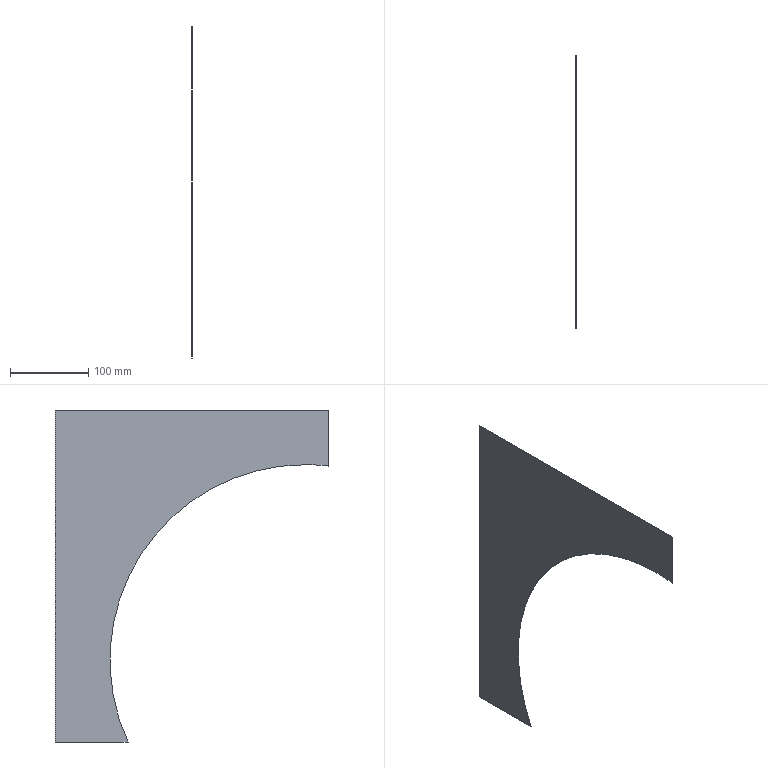Part | STEP file | 09-02 Inner base plate 1 | 1 solid | 8 faces | box 1 x 350 x 425 mm | volume 63574 mm3 | plane 6 | cylinder 2 | commonest cylinder face diameters 500 x2
STEP:
#1=CARTESIAN_POINT('',(0.,0.,0.));
#2=DIRECTION('',(0.,0.,1.));
#3=DIRECTION('',(1.,0.,0.));
#4=AXIS2_PLACEMENT_3D('',#1,#2,#3);
#5=CARTESIAN_POINT('',(0.,256.881,-425.));
#6=VERTEX_POINT('',#5);
#7=CARTESIAN_POINT('',(1.,256.881,-425.));
#8=VERTEX_POINT('',#7);
#9=CARTESIAN_POINT('',(0.5,256.881,-425.));
#10=DIRECTION('',(1.,0.,0.));
#11=VECTOR('',#10,1.);
#12=LINE('',#9,#11);
#13=CARTESIAN_POINT('',(1.,30.,-320.));
#14=DIRECTION('',(-1.,0.,0.));
#15=DIRECTION('',(0.,0.,1.));
#16=AXIS2_PLACEMENT_3D('',#13,#14,#15);
#17=CYLINDRICAL_SURFACE('',#16,250.);
#18=CARTESIAN_POINT('',(2.004,0.5));
#19=DIRECTION('',(0.,-1.));
#20=VECTOR('',#19,1.);
#21=LINE('',#18,#20);
#22=(GEOMETRIC_REPRESENTATION_CONTEXT(2)PARAMETRIC_REPRESENTATION_CONTEXT()REPRESENTATION_CONTEXT('',''));
#23=DEFINITIONAL_REPRESENTATION('',(#21),#22);
#24=PCURVE('',#17,#23);
#25=CARTESIAN_POINT('',(0.,256.881,-425.));
#26=DIRECTION('',(0.,0.,1.));
#27=DIRECTION('',(1.,0.,0.));
#28=AXIS2_PLACEMENT_3D('',#25,#26,#27);
#29=PLANE('',#28);
#30=CARTESIAN_POINT('',(0.5,0.));
#31=DIRECTION('',(1.,0.));
#32=VECTOR('',#31,1.);
#33=LINE('',#30,#32);
#34=(GEOMETRIC_REPRESENTATION_CONTEXT(2)PARAMETRIC_REPRESENTATION_CONTEXT()REPRESENTATION_CONTEXT('',''));
#35=DEFINITIONAL_REPRESENTATION('',(#33),#34);
#36=PCURVE('',#29,#35);
#37=SURFACE_CURVE('',#12,(#24,#36),.PCURVE_S1.);
#38=EDGE_CURVE('',#6,#8,#37,.T.);
#39=ORIENTED_EDGE('',*,*,#38,.F.);
#40=CARTESIAN_POINT('',(0.,30.,-70.));
#41=VERTEX_POINT('',#40);
#42=CARTESIAN_POINT('',(0.,30.,-320.));
#43=DIRECTION('',(-1.,0.,0.));
#44=DIRECTION('',(0.,0.,1.));
#45=AXIS2_PLACEMENT_3D('',#42,#43,#44);
#46=CIRCLE('',#45,250.);
#47=CARTESIAN_POINT('',(0.,1.));
#48=DIRECTION('',(1.,0.));
#49=VECTOR('',#48,1.);
#50=LINE('',#47,#49);
#51=(GEOMETRIC_REPRESENTATION_CONTEXT(2)PARAMETRIC_REPRESENTATION_CONTEXT()REPRESENTATION_CONTEXT('',''));
#52=DEFINITIONAL_REPRESENTATION('',(#50),#51);
#53=PCURVE('',#17,#52);
#54=CARTESIAN_POINT('',(0.,0.,0.));
#55=DIRECTION('',(1.,0.,0.));
#56=DIRECTION('',(0.,0.,-1.));
#57=AXIS2_PLACEMENT_3D('',#54,#55,#56);
#58=PLANE('',#57);
#59=CARTESIAN_POINT('',(70.,30.));
#60=CARTESIAN_POINT('',(70.,463.013));
#61=CARTESIAN_POINT('',(445.,246.506));
#62=CARTESIAN_POINT('',(820.,30.));
#63=CARTESIAN_POINT('',(445.,-186.506));
#64=CARTESIAN_POINT('',(70.,-403.013));
#65=CARTESIAN_POINT('',(70.,30.));
#66=(BOUNDED_CURVE()B_SPLINE_CURVE(2,(#59,#60,#61,#62,#63,#64,#65),.UNSPECIFIED.,.T.,.F.)B_SPLINE_CURVE_WITH_KNOTS((1,2,2,2,2,1),(-2.094,0.,2.094,4.189,6.283,8.378),.UNSPECIFIED.)CURVE()GEOMETRIC_REPRESENTATION_ITEM()RATIONAL_B_SPLINE_CURVE((1.,0.5,1.,0.5,1.,0.5,1.))REPRESENTATION_ITEM(''));
#67=(GEOMETRIC_REPRESENTATION_CONTEXT(2)PARAMETRIC_REPRESENTATION_CONTEXT()REPRESENTATION_CONTEXT('',''));
#68=DEFINITIONAL_REPRESENTATION('',(#66),#67);
#69=PCURVE('',#58,#68);
#70=SURFACE_CURVE('',#46,(#53,#69),.PCURVE_S1.);
#71=EDGE_CURVE('',#41,#6,#70,.T.);
#72=ORIENTED_EDGE('',*,*,#71,.F.);
#73=CARTESIAN_POINT('',(1.,30.,-70.));
#74=VERTEX_POINT('',#73);
#75=CARTESIAN_POINT('',(1.,30.,-70.));
#76=DIRECTION('',(-1.,0.,0.));
#77=VECTOR('',#76,1.);
#78=LINE('',#75,#77);
#79=CARTESIAN_POINT('',(0.,0.));
#80=DIRECTION('',(0.,1.));
#81=VECTOR('',#80,1.);
#82=LINE('',#79,#81);
#83=(GEOMETRIC_REPRESENTATION_CONTEXT(2)PARAMETRIC_REPRESENTATION_CONTEXT()REPRESENTATION_CONTEXT('',''));
#84=DEFINITIONAL_REPRESENTATION('',(#82),#83);
#85=PCURVE('',#17,#84);
#86=CARTESIAN_POINT('',(1.,30.,-320.));
#87=DIRECTION('',(-1.,0.,0.));
#88=DIRECTION('',(0.,0.,1.));
#89=AXIS2_PLACEMENT_3D('',#86,#87,#88);
#90=CYLINDRICAL_SURFACE('',#89,250.);
#91=CARTESIAN_POINT('',(6.283,0.));
#92=DIRECTION('',(0.,1.));
#93=VECTOR('',#92,1.);
#94=LINE('',#91,#93);
#95=(GEOMETRIC_REPRESENTATION_CONTEXT(2)PARAMETRIC_REPRESENTATION_CONTEXT()REPRESENTATION_CONTEXT('',''));
#96=DEFINITIONAL_REPRESENTATION('',(#94),#95);
#97=PCURVE('',#90,#96);
#98=SURFACE_CURVE('',#78,(#85,#97),.PCURVE_S1.);
#99=EDGE_CURVE('',#74,#41,#98,.T.);
#100=ORIENTED_EDGE('',*,*,#99,.F.);
#101=CARTESIAN_POINT('',(1.,30.,-320.));
#102=DIRECTION('',(1.,0.,0.));
#103=DIRECTION('',(0.,0.,1.));
#104=AXIS2_PLACEMENT_3D('',#101,#102,#103);
#105=CIRCLE('',#104,250.);
#106=CARTESIAN_POINT('',(6.283,0.));
#107=DIRECTION('',(-1.,0.));
#108=VECTOR('',#107,1.);
#109=LINE('',#106,#108);
#110=(GEOMETRIC_REPRESENTATION_CONTEXT(2)PARAMETRIC_REPRESENTATION_CONTEXT()REPRESENTATION_CONTEXT('',''));
#111=DEFINITIONAL_REPRESENTATION('',(#109),#110);
#112=PCURVE('',#17,#111);
#113=CARTESIAN_POINT('',(1.,0.,0.));
#114=DIRECTION('',(1.,0.,0.));
#115=DIRECTION('',(0.,0.,-1.));
#116=AXIS2_PLACEMENT_3D('',#113,#114,#115);
#117=PLANE('',#116);
#118=CARTESIAN_POINT('',(320.,30.));
#119=DIRECTION('',(-1.,0.));
#120=AXIS2_PLACEMENT_2D('',#118,#119);
#121=CIRCLE('',#120,250.);
#122=(GEOMETRIC_REPRESENTATION_CONTEXT(2)PARAMETRIC_REPRESENTATION_CONTEXT()REPRESENTATION_CONTEXT('',''));
#123=DEFINITIONAL_REPRESENTATION('',(#121),#122);
#124=PCURVE('',#117,#123);
#125=SURFACE_CURVE('',#105,(#112,#124),.PCURVE_S1.);
#126=EDGE_CURVE('',#8,#74,#125,.T.);
#127=ORIENTED_EDGE('',*,*,#126,.F.);
#128=EDGE_LOOP('',(#39,#72,#100,#127));
#129=FACE_BOUND('',#128,.F.);
#130=ADVANCED_FACE('',(#129),#17,.F.);
#131=CARTESIAN_POINT('',(0.,0.000000027,-71.807));
#132=VERTEX_POINT('',#131);
#133=CARTESIAN_POINT('',(0.,30.,-320.));
#134=DIRECTION('',(-1.,0.,0.));
#135=DIRECTION('',(0.,0.,1.));
#136=AXIS2_PLACEMENT_3D('',#133,#134,#135);
#137=CIRCLE('',#136,250.);
#138=CARTESIAN_POINT('',(0.,1.));
#139=DIRECTION('',(1.,0.));
#140=VECTOR('',#139,1.);
#141=LINE('',#138,#140);
#142=(GEOMETRIC_REPRESENTATION_CONTEXT(2)PARAMETRIC_REPRESENTATION_CONTEXT()REPRESENTATION_CONTEXT('',''));
#143=DEFINITIONAL_REPRESENTATION('',(#141),#142);
#144=PCURVE('',#90,#143);
#145=CARTESIAN_POINT('',(70.,30.));
#146=CARTESIAN_POINT('',(70.,463.013));
#147=CARTESIAN_POINT('',(445.,246.506));
#148=CARTESIAN_POINT('',(820.,30.));
#149=CARTESIAN_POINT('',(445.,-186.506));
#150=CARTESIAN_POINT('',(70.,-403.013));
#151=CARTESIAN_POINT('',(70.,30.));
#152=(BOUNDED_CURVE()B_SPLINE_CURVE(2,(#145,#146,#147,#148,#149,#150,#151),.UNSPECIFIED.,.T.,.F.)B_SPLINE_CURVE_WITH_KNOTS((1,2,2,2,2,1),(-2.094,0.,2.094,4.189,6.283,8.378),.UNSPECIFIED.)CURVE()GEOMETRIC_REPRESENTATION_ITEM()RATIONAL_B_SPLINE_CURVE((1.,0.5,1.,0.5,1.,0.5,1.))REPRESENTATION_ITEM(''));
#153=(GEOMETRIC_REPRESENTATION_CONTEXT(2)PARAMETRIC_REPRESENTATION_CONTEXT()REPRESENTATION_CONTEXT('',''));
#154=DEFINITIONAL_REPRESENTATION('',(#152),#153);
#155=PCURVE('',#58,#154);
#156=SURFACE_CURVE('',#137,(#144,#155),.PCURVE_S1.);
#157=EDGE_CURVE('',#132,#41,#156,.T.);
#158=ORIENTED_EDGE('',*,*,#157,.F.);
#159=CARTESIAN_POINT('',(1.,0.000000027,-71.807));
#160=VERTEX_POINT('',#159);
#161=CARTESIAN_POINT('',(0.5,0.000000053,-71.807));
#162=DIRECTION('',(-1.,0.,0.));
#163=VECTOR('',#162,1.);
#164=LINE('',#161,#163);
#165=CARTESIAN_POINT('',(6.163,0.5));
#166=DIRECTION('',(0.,1.));
#167=VECTOR('',#166,1.);
#168=LINE('',#165,#167);
#169=(GEOMETRIC_REPRESENTATION_CONTEXT(2)PARAMETRIC_REPRESENTATION_CONTEXT()REPRESENTATION_CONTEXT('',''));
#170=DEFINITIONAL_REPRESENTATION('',(#168),#169);
#171=PCURVE('',#90,#170);
#172=CARTESIAN_POINT('',(0.,0.,-71.807));
#173=DIRECTION('',(0.,1.,0.));
#174=DIRECTION('',(0.,0.,1.));
#175=AXIS2_PLACEMENT_3D('',#172,#173,#174);
#176=PLANE('',#175);
#177=CARTESIAN_POINT('',(0.000000006,0.5));
#178=DIRECTION('',(0.,-1.));
#179=VECTOR('',#178,1.);
#180=LINE('',#177,#179);
#181=(GEOMETRIC_REPRESENTATION_CONTEXT(2)PARAMETRIC_REPRESENTATION_CONTEXT()REPRESENTATION_CONTEXT('',''));
#182=DEFINITIONAL_REPRESENTATION('',(#180),#181);
#183=PCURVE('',#176,#182);
#184=SURFACE_CURVE('',#164,(#171,#183),.PCURVE_S1.);
#185=EDGE_CURVE('',#160,#132,#184,.T.);
#186=ORIENTED_EDGE('',*,*,#185,.F.);
#187=CARTESIAN_POINT('',(1.,30.,-320.));
#188=DIRECTION('',(1.,0.,0.));
#189=DIRECTION('',(0.,0.,1.));
#190=AXIS2_PLACEMENT_3D('',#187,#188,#189);
#191=CIRCLE('',#190,250.);
#192=CARTESIAN_POINT('',(6.283,0.));
#193=DIRECTION('',(-1.,0.));
#194=VECTOR('',#193,1.);
#195=LINE('',#192,#194);
#196=(GEOMETRIC_REPRESENTATION_CONTEXT(2)PARAMETRIC_REPRESENTATION_CONTEXT()REPRESENTATION_CONTEXT('',''));
#197=DEFINITIONAL_REPRESENTATION('',(#195),#196);
#198=PCURVE('',#90,#197);
#199=CARTESIAN_POINT('',(320.,30.));
#200=DIRECTION('',(-1.,0.));
#201=AXIS2_PLACEMENT_2D('',#199,#200);
#202=CIRCLE('',#201,250.);
#203=(GEOMETRIC_REPRESENTATION_CONTEXT(2)PARAMETRIC_REPRESENTATION_CONTEXT()REPRESENTATION_CONTEXT('',''));
#204=DEFINITIONAL_REPRESENTATION('',(#202),#203);
#205=PCURVE('',#117,#204);
#206=SURFACE_CURVE('',#191,(#198,#205),.PCURVE_S1.);
#207=EDGE_CURVE('',#74,#160,#206,.T.);
#208=ORIENTED_EDGE('',*,*,#207,.F.);
#209=ORIENTED_EDGE('',*,*,#99,.T.);
#210=EDGE_LOOP('',(#158,#186,#208,#209));
#211=FACE_BOUND('',#210,.F.);
#212=ADVANCED_FACE('',(#211),#90,.F.);
#213=CARTESIAN_POINT('',(0.,350.,-425.));
#214=VERTEX_POINT('',#213);
#215=CARTESIAN_POINT('',(0.,350.,0.));
#216=VERTEX_POINT('',#215);
#217=CARTESIAN_POINT('',(0.,350.,-212.5));
#218=DIRECTION('',(0.,0.,1.));
#219=VECTOR('',#218,1.);
#220=LINE('',#217,#219);
#221=CARTESIAN_POINT('',(212.5,350.));
#222=DIRECTION('',(-1.,0.));
#223=VECTOR('',#222,1.);
#224=LINE('',#221,#223);
#225=(GEOMETRIC_REPRESENTATION_CONTEXT(2)PARAMETRIC_REPRESENTATION_CONTEXT()REPRESENTATION_CONTEXT('',''));
#226=DEFINITIONAL_REPRESENTATION('',(#224),#225);
#227=PCURVE('',#58,#226);
#228=CARTESIAN_POINT('',(0.,350.,0.));
#229=DIRECTION('',(0.,-1.,0.));
#230=DIRECTION('',(0.,0.,-1.));
#231=AXIS2_PLACEMENT_3D('',#228,#229,#230);
#232=PLANE('',#231);
#233=CARTESIAN_POINT('',(212.5,0.));
#234=DIRECTION('',(-1.,0.));
#235=VECTOR('',#234,1.);
#236=LINE('',#233,#235);
#237=(GEOMETRIC_REPRESENTATION_CONTEXT(2)PARAMETRIC_REPRESENTATION_CONTEXT()REPRESENTATION_CONTEXT('',''));
#238=DEFINITIONAL_REPRESENTATION('',(#236),#237);
#239=PCURVE('',#232,#238);
#240=SURFACE_CURVE('',#220,(#227,#239),.PCURVE_S1.);
#241=EDGE_CURVE('',#214,#216,#240,.T.);
#242=ORIENTED_EDGE('',*,*,#241,.F.);
#243=CARTESIAN_POINT('',(0.,175.,-425.));
#244=DIRECTION('',(0.,1.,0.));
#245=VECTOR('',#244,1.);
#246=LINE('',#243,#245);
#247=CARTESIAN_POINT('',(425.,175.));
#248=DIRECTION('',(0.,1.));
#249=VECTOR('',#248,1.);
#250=LINE('',#247,#249);
#251=(GEOMETRIC_REPRESENTATION_CONTEXT(2)PARAMETRIC_REPRESENTATION_CONTEXT()REPRESENTATION_CONTEXT('',''));
#252=DEFINITIONAL_REPRESENTATION('',(#250),#251);
#253=PCURVE('',#58,#252);
#254=CARTESIAN_POINT('',(0.,-81.881));
#255=DIRECTION('',(0.,1.));
#256=VECTOR('',#255,1.);
#257=LINE('',#254,#256);
#258=(GEOMETRIC_REPRESENTATION_CONTEXT(2)PARAMETRIC_REPRESENTATION_CONTEXT()REPRESENTATION_CONTEXT('',''));
#259=DEFINITIONAL_REPRESENTATION('',(#257),#258);
#260=PCURVE('',#29,#259);
#261=SURFACE_CURVE('',#246,(#253,#260),.PCURVE_S1.);
#262=EDGE_CURVE('',#6,#214,#261,.T.);
#263=ORIENTED_EDGE('',*,*,#262,.F.);
#264=ORIENTED_EDGE('',*,*,#71,.F.);
#265=ORIENTED_EDGE('',*,*,#157,.F.);
#266=CARTESIAN_POINT('',(0.,0.,0.));
#267=VERTEX_POINT('',#266);
#268=CARTESIAN_POINT('',(0.,0.,-212.5));
#269=DIRECTION('',(0.,0.,-1.));
#270=VECTOR('',#269,1.);
#271=LINE('',#268,#270);
#272=CARTESIAN_POINT('',(212.5,0.));
#273=DIRECTION('',(1.,0.));
#274=VECTOR('',#273,1.);
#275=LINE('',#272,#274);
#276=(GEOMETRIC_REPRESENTATION_CONTEXT(2)PARAMETRIC_REPRESENTATION_CONTEXT()REPRESENTATION_CONTEXT('',''));
#277=DEFINITIONAL_REPRESENTATION('',(#275),#276);
#278=PCURVE('',#58,#277);
#279=CARTESIAN_POINT('',(-140.693,0.));
#280=DIRECTION('',(-1.,0.));
#281=VECTOR('',#280,1.);
#282=LINE('',#279,#281);
#283=(GEOMETRIC_REPRESENTATION_CONTEXT(2)PARAMETRIC_REPRESENTATION_CONTEXT()REPRESENTATION_CONTEXT('',''));
#284=DEFINITIONAL_REPRESENTATION('',(#282),#283);
#285=PCURVE('',#176,#284);
#286=SURFACE_CURVE('',#271,(#278,#285),.PCURVE_S1.);
#287=EDGE_CURVE('',#267,#132,#286,.T.);
#288=ORIENTED_EDGE('',*,*,#287,.F.);
#289=CARTESIAN_POINT('',(0.,175.,0.));
#290=DIRECTION('',(0.,-1.,0.));
#291=VECTOR('',#290,1.);
#292=LINE('',#289,#291);
#293=CARTESIAN_POINT('',(0.,175.));
#294=DIRECTION('',(0.,-1.));
#295=VECTOR('',#294,1.);
#296=LINE('',#293,#295);
#297=(GEOMETRIC_REPRESENTATION_CONTEXT(2)PARAMETRIC_REPRESENTATION_CONTEXT()REPRESENTATION_CONTEXT('',''));
#298=DEFINITIONAL_REPRESENTATION('',(#296),#297);
#299=PCURVE('',#58,#298);
#300=CARTESIAN_POINT('',(1.,0.,0.));
#301=DIRECTION('',(0.,0.,-1.));
#302=DIRECTION('',(-1.,0.,0.));
#303=AXIS2_PLACEMENT_3D('',#300,#301,#302);
#304=PLANE('',#303);
#305=CARTESIAN_POINT('',(1.,175.));
#306=DIRECTION('',(0.,-1.));
#307=VECTOR('',#306,1.);
#308=LINE('',#305,#307);
#309=(GEOMETRIC_REPRESENTATION_CONTEXT(2)PARAMETRIC_REPRESENTATION_CONTEXT()REPRESENTATION_CONTEXT('',''));
#310=DEFINITIONAL_REPRESENTATION('',(#308),#309);
#311=PCURVE('',#304,#310);
#312=SURFACE_CURVE('',#292,(#299,#311),.PCURVE_S1.);
#313=EDGE_CURVE('',#216,#267,#312,.T.);
#314=ORIENTED_EDGE('',*,*,#313,.F.);
#315=EDGE_LOOP('',(#242,#263,#264,#265,#288,#314));
#316=FACE_BOUND('',#315,.T.);
#317=ADVANCED_FACE('',(#316),#58,.F.);
#318=CARTESIAN_POINT('',(1.,350.,-425.));
#319=VERTEX_POINT('',#318);
#320=CARTESIAN_POINT('',(1.,175.,-425.));
#321=DIRECTION('',(0.,1.,0.));
#322=VECTOR('',#321,1.);
#323=LINE('',#320,#322);
#324=CARTESIAN_POINT('',(425.,175.));
#325=DIRECTION('',(0.,1.));
#326=VECTOR('',#325,1.);
#327=LINE('',#324,#326);
#328=(GEOMETRIC_REPRESENTATION_CONTEXT(2)PARAMETRIC_REPRESENTATION_CONTEXT()REPRESENTATION_CONTEXT('',''));
#329=DEFINITIONAL_REPRESENTATION('',(#327),#328);
#330=PCURVE('',#117,#329);
#331=CARTESIAN_POINT('',(1.,-81.881));
#332=DIRECTION('',(0.,1.));
#333=VECTOR('',#332,1.);
#334=LINE('',#331,#333);
#335=(GEOMETRIC_REPRESENTATION_CONTEXT(2)PARAMETRIC_REPRESENTATION_CONTEXT()REPRESENTATION_CONTEXT('',''));
#336=DEFINITIONAL_REPRESENTATION('',(#334),#335);
#337=PCURVE('',#29,#336);
#338=SURFACE_CURVE('',#323,(#330,#337),.PCURVE_S1.);
#339=EDGE_CURVE('',#8,#319,#338,.T.);
#340=ORIENTED_EDGE('',*,*,#339,.T.);
#341=CARTESIAN_POINT('',(1.,350.,0.));
#342=VERTEX_POINT('',#341);
#343=CARTESIAN_POINT('',(1.,350.,-212.5));
#344=DIRECTION('',(0.,0.,1.));
#345=VECTOR('',#344,1.);
#346=LINE('',#343,#345);
#347=CARTESIAN_POINT('',(212.5,350.));
#348=DIRECTION('',(-1.,0.));
#349=VECTOR('',#348,1.);
#350=LINE('',#347,#349);
#351=(GEOMETRIC_REPRESENTATION_CONTEXT(2)PARAMETRIC_REPRESENTATION_CONTEXT()REPRESENTATION_CONTEXT('',''));
#352=DEFINITIONAL_REPRESENTATION('',(#350),#351);
#353=PCURVE('',#117,#352);
#354=CARTESIAN_POINT('',(212.5,1.));
#355=DIRECTION('',(-1.,0.));
#356=VECTOR('',#355,1.);
#357=LINE('',#354,#356);
#358=(GEOMETRIC_REPRESENTATION_CONTEXT(2)PARAMETRIC_REPRESENTATION_CONTEXT()REPRESENTATION_CONTEXT('',''));
#359=DEFINITIONAL_REPRESENTATION('',(#357),#358);
#360=PCURVE('',#232,#359);
#361=SURFACE_CURVE('',#346,(#353,#360),.PCURVE_S1.);
#362=EDGE_CURVE('',#319,#342,#361,.T.);
#363=ORIENTED_EDGE('',*,*,#362,.T.);
#364=CARTESIAN_POINT('',(1.,0.,0.));
#365=VERTEX_POINT('',#364);
#366=CARTESIAN_POINT('',(1.,175.,0.));
#367=DIRECTION('',(0.,-1.,0.));
#368=VECTOR('',#367,1.);
#369=LINE('',#366,#368);
#370=CARTESIAN_POINT('',(0.,175.));
#371=DIRECTION('',(0.,-1.));
#372=VECTOR('',#371,1.);
#373=LINE('',#370,#372);
#374=(GEOMETRIC_REPRESENTATION_CONTEXT(2)PARAMETRIC_REPRESENTATION_CONTEXT()REPRESENTATION_CONTEXT('',''));
#375=DEFINITIONAL_REPRESENTATION('',(#373),#374);
#376=PCURVE('',#117,#375);
#377=CARTESIAN_POINT('',(0.,175.));
#378=DIRECTION('',(0.,-1.));
#379=VECTOR('',#378,1.);
#380=LINE('',#377,#379);
#381=(GEOMETRIC_REPRESENTATION_CONTEXT(2)PARAMETRIC_REPRESENTATION_CONTEXT()REPRESENTATION_CONTEXT('',''));
#382=DEFINITIONAL_REPRESENTATION('',(#380),#381);
#383=PCURVE('',#304,#382);
#384=SURFACE_CURVE('',#369,(#376,#383),.PCURVE_S1.);
#385=EDGE_CURVE('',#342,#365,#384,.T.);
#386=ORIENTED_EDGE('',*,*,#385,.T.);
#387=CARTESIAN_POINT('',(1.,0.,-212.5));
#388=DIRECTION('',(0.,0.,-1.));
#389=VECTOR('',#388,1.);
#390=LINE('',#387,#389);
#391=CARTESIAN_POINT('',(212.5,0.));
#392=DIRECTION('',(1.,0.));
#393=VECTOR('',#392,1.);
#394=LINE('',#391,#393);
#395=(GEOMETRIC_REPRESENTATION_CONTEXT(2)PARAMETRIC_REPRESENTATION_CONTEXT()REPRESENTATION_CONTEXT('',''));
#396=DEFINITIONAL_REPRESENTATION('',(#394),#395);
#397=PCURVE('',#117,#396);
#398=CARTESIAN_POINT('',(-140.693,1.));
#399=DIRECTION('',(-1.,0.));
#400=VECTOR('',#399,1.);
#401=LINE('',#398,#400);
#402=(GEOMETRIC_REPRESENTATION_CONTEXT(2)PARAMETRIC_REPRESENTATION_CONTEXT()REPRESENTATION_CONTEXT('',''));
#403=DEFINITIONAL_REPRESENTATION('',(#401),#402);
#404=PCURVE('',#176,#403);
#405=SURFACE_CURVE('',#390,(#397,#404),.PCURVE_S1.);
#406=EDGE_CURVE('',#365,#160,#405,.T.);
#407=ORIENTED_EDGE('',*,*,#406,.T.);
#408=ORIENTED_EDGE('',*,*,#207,.F.);
#409=ORIENTED_EDGE('',*,*,#126,.F.);
#410=EDGE_LOOP('',(#340,#363,#386,#407,#408,#409));
#411=FACE_BOUND('',#410,.T.);
#412=ADVANCED_FACE('',(#411),#117,.T.);
#413=CARTESIAN_POINT('',(0.5,0.,0.));
#414=DIRECTION('',(-1.,0.,0.));
#415=VECTOR('',#414,1.);
#416=LINE('',#413,#415);
#417=CARTESIAN_POINT('',(0.5,0.));
#418=DIRECTION('',(1.,0.));
#419=VECTOR('',#418,1.);
#420=LINE('',#417,#419);
#421=(GEOMETRIC_REPRESENTATION_CONTEXT(2)PARAMETRIC_REPRESENTATION_CONTEXT()REPRESENTATION_CONTEXT('',''));
#422=DEFINITIONAL_REPRESENTATION('',(#420),#421);
#423=PCURVE('',#304,#422);
#424=CARTESIAN_POINT('',(71.807,0.5));
#425=DIRECTION('',(0.,-1.));
#426=VECTOR('',#425,1.);
#427=LINE('',#424,#426);
#428=(GEOMETRIC_REPRESENTATION_CONTEXT(2)PARAMETRIC_REPRESENTATION_CONTEXT()REPRESENTATION_CONTEXT('',''));
#429=DEFINITIONAL_REPRESENTATION('',(#427),#428);
#430=PCURVE('',#176,#429);
#431=SURFACE_CURVE('',#416,(#423,#430),.PCURVE_S1.);
#432=EDGE_CURVE('',#365,#267,#431,.T.);
#433=ORIENTED_EDGE('',*,*,#432,.F.);
#434=ORIENTED_EDGE('',*,*,#385,.F.);
#435=CARTESIAN_POINT('',(0.5,350.,0.));
#436=DIRECTION('',(1.,0.,0.));
#437=VECTOR('',#436,1.);
#438=LINE('',#435,#437);
#439=CARTESIAN_POINT('',(0.5,350.));
#440=DIRECTION('',(-1.,0.));
#441=VECTOR('',#440,1.);
#442=LINE('',#439,#441);
#443=(GEOMETRIC_REPRESENTATION_CONTEXT(2)PARAMETRIC_REPRESENTATION_CONTEXT()REPRESENTATION_CONTEXT('',''));
#444=DEFINITIONAL_REPRESENTATION('',(#442),#443);
#445=PCURVE('',#304,#444);
#446=CARTESIAN_POINT('',(0.,0.5));
#447=DIRECTION('',(0.,1.));
#448=VECTOR('',#447,1.);
#449=LINE('',#446,#448);
#450=(GEOMETRIC_REPRESENTATION_CONTEXT(2)PARAMETRIC_REPRESENTATION_CONTEXT()REPRESENTATION_CONTEXT('',''));
#451=DEFINITIONAL_REPRESENTATION('',(#449),#450);
#452=PCURVE('',#232,#451);
#453=SURFACE_CURVE('',#438,(#445,#452),.PCURVE_S1.);
#454=EDGE_CURVE('',#216,#342,#453,.T.);
#455=ORIENTED_EDGE('',*,*,#454,.F.);
#456=ORIENTED_EDGE('',*,*,#313,.T.);
#457=EDGE_LOOP('',(#433,#434,#455,#456));
#458=FACE_BOUND('',#457,.T.);
#459=ADVANCED_FACE('',(#458),#304,.F.);
#460=ORIENTED_EDGE('',*,*,#454,.T.);
#461=ORIENTED_EDGE('',*,*,#362,.F.);
#462=CARTESIAN_POINT('',(0.5,350.,-425.));
#463=DIRECTION('',(1.,0.,0.));
#464=VECTOR('',#463,1.);
#465=LINE('',#462,#464);
#466=CARTESIAN_POINT('',(425.,0.5));
#467=DIRECTION('',(0.,1.));
#468=VECTOR('',#467,1.);
#469=LINE('',#466,#468);
#470=(GEOMETRIC_REPRESENTATION_CONTEXT(2)PARAMETRIC_REPRESENTATION_CONTEXT()REPRESENTATION_CONTEXT('',''));
#471=DEFINITIONAL_REPRESENTATION('',(#469),#470);
#472=PCURVE('',#232,#471);
#473=CARTESIAN_POINT('',(0.5,93.119));
#474=DIRECTION('',(1.,0.));
#475=VECTOR('',#474,1.);
#476=LINE('',#473,#475);
#477=(GEOMETRIC_REPRESENTATION_CONTEXT(2)PARAMETRIC_REPRESENTATION_CONTEXT()REPRESENTATION_CONTEXT('',''));
#478=DEFINITIONAL_REPRESENTATION('',(#476),#477);
#479=PCURVE('',#29,#478);
#480=SURFACE_CURVE('',#465,(#472,#479),.PCURVE_S1.);
#481=EDGE_CURVE('',#214,#319,#480,.T.);
#482=ORIENTED_EDGE('',*,*,#481,.F.);
#483=ORIENTED_EDGE('',*,*,#241,.T.);
#484=EDGE_LOOP('',(#460,#461,#482,#483));
#485=FACE_BOUND('',#484,.T.);
#486=ADVANCED_FACE('',(#485),#232,.F.);
#487=ORIENTED_EDGE('',*,*,#481,.T.);
#488=ORIENTED_EDGE('',*,*,#339,.F.);
#489=ORIENTED_EDGE('',*,*,#38,.F.);
#490=ORIENTED_EDGE('',*,*,#262,.T.);
#491=EDGE_LOOP('',(#487,#488,#489,#490));
#492=FACE_BOUND('',#491,.T.);
#493=ADVANCED_FACE('',(#492),#29,.F.);
#494=ORIENTED_EDGE('',*,*,#185,.F.);
#495=ORIENTED_EDGE('',*,*,#406,.F.);
#496=ORIENTED_EDGE('',*,*,#432,.T.);
#497=ORIENTED_EDGE('',*,*,#287,.T.);
#498=EDGE_LOOP('',(#494,#495,#496,#497));
#499=FACE_BOUND('',#498,.T.);
#500=ADVANCED_FACE('',(#499),#176,.F.);
#501=CLOSED_SHELL('',(#130,#212,#317,#412,#459,#486,#493,#500));
#502=MANIFOLD_SOLID_BREP('',#501);
#503=(LENGTH_UNIT()NAMED_UNIT(*)SI_UNIT(.MILLI.,.METRE.));
#504=UNCERTAINTY_MEASURE_WITH_UNIT(LENGTH_MEASURE(0.0000001),#503,'','');
#505=(NAMED_UNIT(*)PLANE_ANGLE_UNIT()SI_UNIT($,.RADIAN.));
#506=(NAMED_UNIT(*)SI_UNIT($,.STERADIAN.)SOLID_ANGLE_UNIT());
#507=(GEOMETRIC_REPRESENTATION_CONTEXT(3)GLOBAL_UNCERTAINTY_ASSIGNED_CONTEXT((#504))GLOBAL_UNIT_ASSIGNED_CONTEXT((#503,#505,#506))REPRESENTATION_CONTEXT('',''));
#508=ADVANCED_BREP_SHAPE_REPRESENTATION('',(#4,#502),#507);